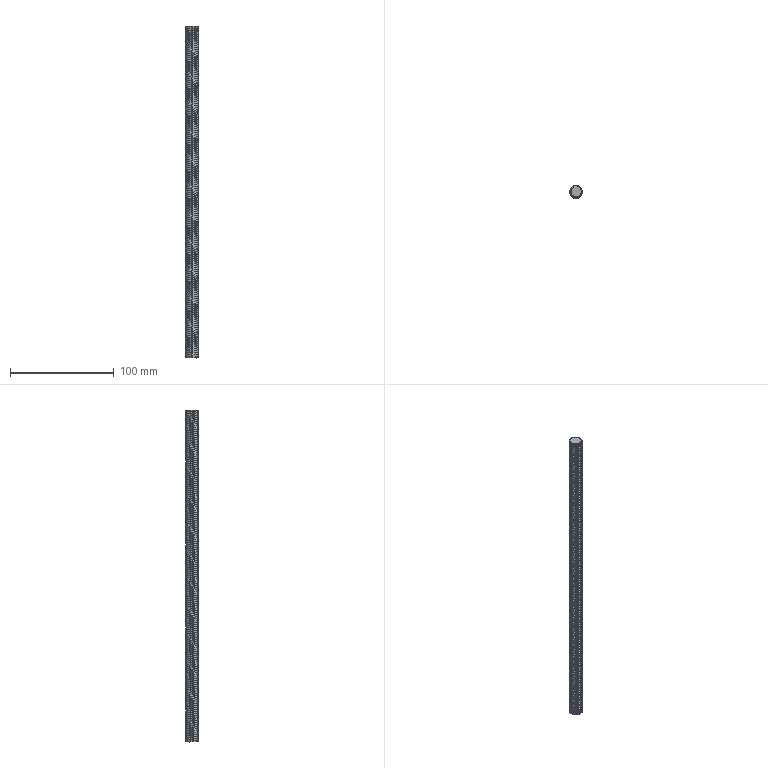Part | STEP file | 1 solid | 326 faces | box 12 x 12 x 320 mm | volume 33018 mm3 | cylinder 322 | spline 2 | plane 2 | commonest cylinder face diameters 12 x322